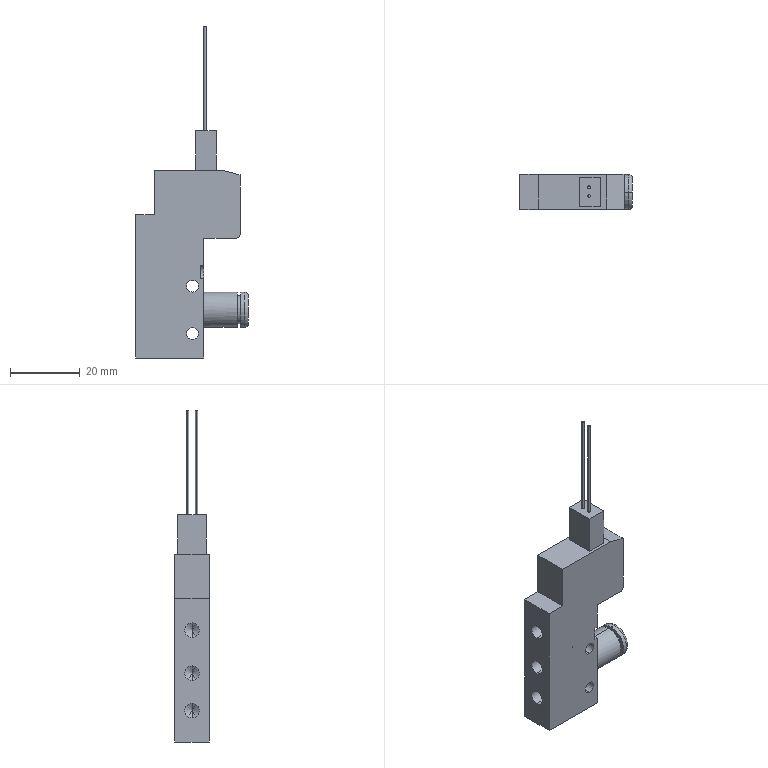Part | SolidWorks | features ICE 8, Fillet 2, 3DProfileFeature 1, Chamfer 1, Extrusion 1, HoleWzd 1, RevCut 1 | 1 solid | 68 faces | box 32.3 x 10 x 95.1 mm | volume 12247 mm3 | plane 31 | cylinder 29 | cone 6 | torus 2 | commonest cylinder face diameters 4.2 x6 0.75 x4 3.4 x4 3.5 x4 10 x4 4 x2